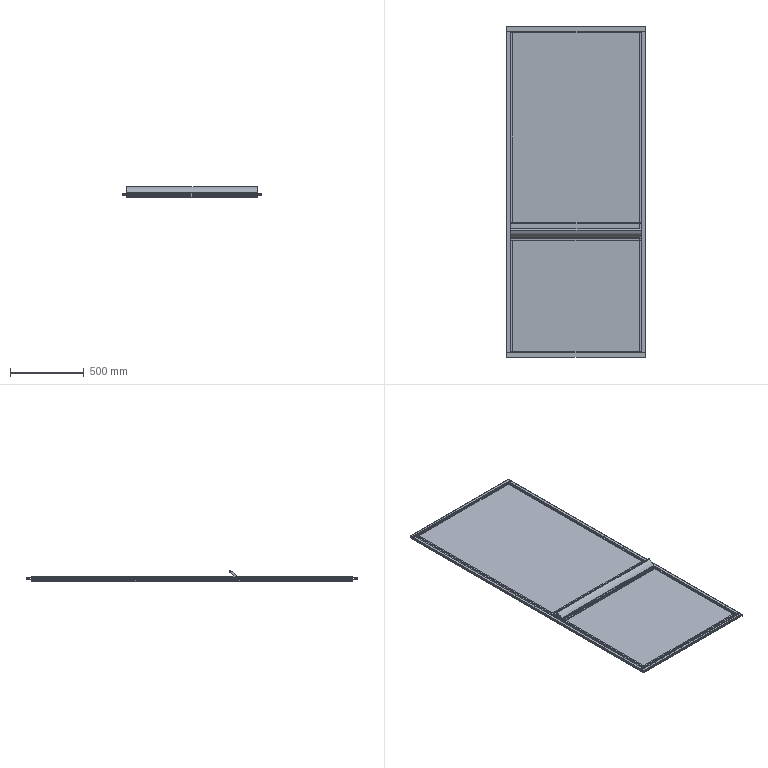Part | SolidWorks | features ICE 13, MirrorSolid 3, LPattern 1, WeldMemberFeat 1, WeldmentFeature 1 | 22 solids | 546 faces | box 940 x 2236 x 71.386 mm | volume 44387536 mm3 | plane 390 | cylinder 156 | commonest cylinder face diameters 1.1 x36 3.6 x32 5.8 x29 4 x24 1 x10 0.4 x8